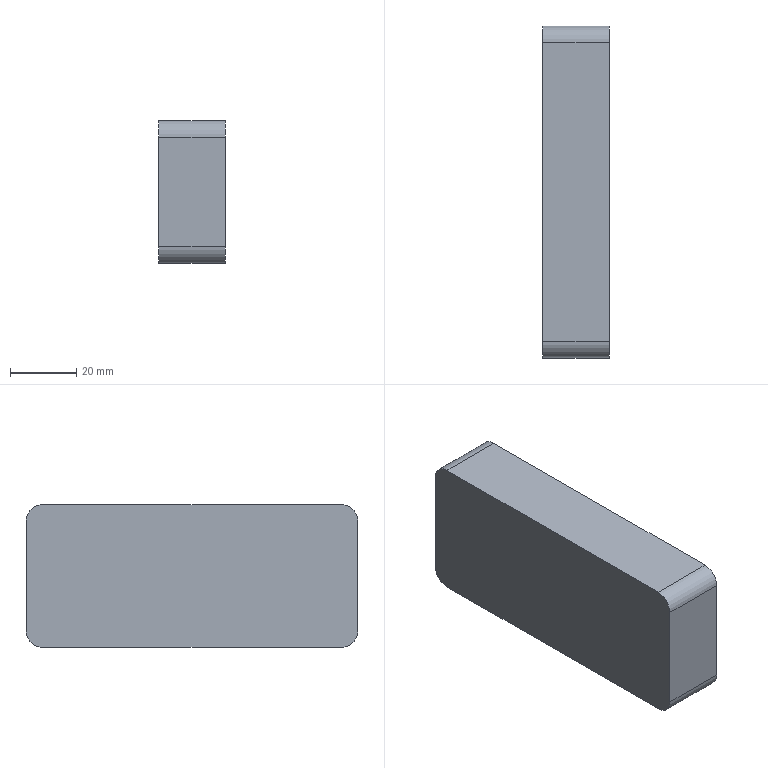Part | STEP file | 4-20.sldasm-Part-14 | 1 solid | 10 faces | box 20 x 100 x 43 mm | volume 85571 mm3 | plane 6 | cylinder 4 | commonest cylinder face diameters 10 x4
STEP:
#1=CARTESIAN_POINT('',(245.,464.25,-67.75));
#2=VERTEX_POINT('',#1);
#3=CARTESIAN_POINT('',(245.,374.25,-67.75));
#4=VERTEX_POINT('',#3);
#5=CARTESIAN_POINT('',(245.,464.25,-67.75));
#6=DIRECTION('',(0.,-1.,0.));
#7=VECTOR('',#6,1000.);
#8=LINE('',#5,#7);
#9=EDGE_CURVE('',#2,#4,#8,.T.);
#10=ORIENTED_EDGE('',*,*,#9,.T.);
#11=CARTESIAN_POINT('',(225.,374.25,-67.75));
#12=VERTEX_POINT('',#11);
#13=CARTESIAN_POINT('',(225.,374.25,-67.75));
#14=DIRECTION('',(1.,0.,0.));
#15=VECTOR('',#14,1000.);
#16=LINE('',#13,#15);
#17=EDGE_CURVE('',#12,#4,#16,.T.);
#18=ORIENTED_EDGE('',*,*,#17,.F.);
#19=CARTESIAN_POINT('',(225.,464.25,-67.75));
#20=VERTEX_POINT('',#19);
#21=CARTESIAN_POINT('',(225.,464.25,-67.75));
#22=DIRECTION('',(0.,-1.,0.));
#23=VECTOR('',#22,1000.);
#24=LINE('',#21,#23);
#25=EDGE_CURVE('',#20,#12,#24,.T.);
#26=ORIENTED_EDGE('',*,*,#25,.F.);
#27=CARTESIAN_POINT('',(225.,464.25,-67.75));
#28=DIRECTION('',(1.,0.,0.));
#29=VECTOR('',#28,1000.);
#30=LINE('',#27,#29);
#31=EDGE_CURVE('',#20,#2,#30,.T.);
#32=ORIENTED_EDGE('',*,*,#31,.T.);
#33=EDGE_LOOP('',(#10,#18,#26,#32));
#34=FACE_OUTER_BOUND('',#33,.T.);
#35=CARTESIAN_POINT('',(225.,464.25,-67.75));
#36=DIRECTION('',(0.,0.,1.));
#37=DIRECTION('',(0.,-1.,0.));
#38=AXIS2_PLACEMENT_3D('',#35,#36,#37);
#39=PLANE('',#38);
#40=ADVANCED_FACE('',(#34),#39,.F.);
#41=CARTESIAN_POINT('',(245.,369.25,-62.75));
#42=VERTEX_POINT('',#41);
#43=CARTESIAN_POINT('',(245.,374.25,-62.75));
#44=DIRECTION('',(-1.,0.,0.));
#45=DIRECTION('',(0.,0.,1.));
#46=AXIS2_PLACEMENT_3D('',#43,#44,#45);
#47=CIRCLE('',#46,5.);
#48=EDGE_CURVE('',#4,#42,#47,.T.);
#49=ORIENTED_EDGE('',*,*,#48,.T.);
#50=CARTESIAN_POINT('',(225.,369.25,-62.75));
#51=VERTEX_POINT('',#50);
#52=CARTESIAN_POINT('',(225.,369.25,-62.75));
#53=DIRECTION('',(1.,0.,0.));
#54=VECTOR('',#53,1000.);
#55=LINE('',#52,#54);
#56=EDGE_CURVE('',#51,#42,#55,.T.);
#57=ORIENTED_EDGE('',*,*,#56,.F.);
#58=CARTESIAN_POINT('',(225.,374.25,-62.75));
#59=DIRECTION('',(-1.,0.,0.));
#60=DIRECTION('',(0.,0.,1.));
#61=AXIS2_PLACEMENT_3D('',#58,#59,#60);
#62=CIRCLE('',#61,5.);
#63=EDGE_CURVE('',#12,#51,#62,.T.);
#64=ORIENTED_EDGE('',*,*,#63,.F.);
#65=ORIENTED_EDGE('',*,*,#17,.T.);
#66=EDGE_LOOP('',(#49,#57,#64,#65));
#67=FACE_OUTER_BOUND('',#66,.T.);
#68=CARTESIAN_POINT('',(225.,374.25,-62.75));
#69=DIRECTION('',(1.,0.,0.));
#70=DIRECTION('',(0.,1.,0.));
#71=AXIS2_PLACEMENT_3D('',#68,#69,#70);
#72=CYLINDRICAL_SURFACE('',#71,5.);
#73=ADVANCED_FACE('',(#67),#72,.T.);
#74=CARTESIAN_POINT('',(245.,369.25,-29.75));
#75=VERTEX_POINT('',#74);
#76=CARTESIAN_POINT('',(245.,369.25,-62.75));
#77=DIRECTION('',(0.,0.,1.));
#78=VECTOR('',#77,1000.);
#79=LINE('',#76,#78);
#80=EDGE_CURVE('',#42,#75,#79,.T.);
#81=ORIENTED_EDGE('',*,*,#80,.T.);
#82=CARTESIAN_POINT('',(225.,369.25,-29.75));
#83=VERTEX_POINT('',#82);
#84=CARTESIAN_POINT('',(225.,369.25,-29.75));
#85=DIRECTION('',(1.,0.,0.));
#86=VECTOR('',#85,1000.);
#87=LINE('',#84,#86);
#88=EDGE_CURVE('',#83,#75,#87,.T.);
#89=ORIENTED_EDGE('',*,*,#88,.F.);
#90=CARTESIAN_POINT('',(225.,369.25,-62.75));
#91=DIRECTION('',(0.,0.,1.));
#92=VECTOR('',#91,1000.);
#93=LINE('',#90,#92);
#94=EDGE_CURVE('',#51,#83,#93,.T.);
#95=ORIENTED_EDGE('',*,*,#94,.F.);
#96=ORIENTED_EDGE('',*,*,#56,.T.);
#97=EDGE_LOOP('',(#81,#89,#95,#96));
#98=FACE_OUTER_BOUND('',#97,.T.);
#99=CARTESIAN_POINT('',(225.,369.25,-62.75));
#100=DIRECTION('',(0.,1.,0.));
#101=DIRECTION('',(-1.,0.,0.));
#102=AXIS2_PLACEMENT_3D('',#99,#100,#101);
#103=PLANE('',#102);
#104=ADVANCED_FACE('',(#98),#103,.F.);
#105=CARTESIAN_POINT('',(245.,374.25,-24.75));
#106=VERTEX_POINT('',#105);
#107=CARTESIAN_POINT('',(245.,374.25,-29.75));
#108=DIRECTION('',(-1.,0.,0.));
#109=DIRECTION('',(0.,0.,1.));
#110=AXIS2_PLACEMENT_3D('',#107,#108,#109);
#111=CIRCLE('',#110,5.);
#112=EDGE_CURVE('',#75,#106,#111,.T.);
#113=ORIENTED_EDGE('',*,*,#112,.T.);
#114=CARTESIAN_POINT('',(225.,374.25,-24.75));
#115=VERTEX_POINT('',#114);
#116=CARTESIAN_POINT('',(225.,374.25,-24.75));
#117=DIRECTION('',(1.,0.,0.));
#118=VECTOR('',#117,1000.);
#119=LINE('',#116,#118);
#120=EDGE_CURVE('',#115,#106,#119,.T.);
#121=ORIENTED_EDGE('',*,*,#120,.F.);
#122=CARTESIAN_POINT('',(225.,374.25,-29.75));
#123=DIRECTION('',(-1.,0.,0.));
#124=DIRECTION('',(0.,0.,1.));
#125=AXIS2_PLACEMENT_3D('',#122,#123,#124);
#126=CIRCLE('',#125,5.);
#127=EDGE_CURVE('',#83,#115,#126,.T.);
#128=ORIENTED_EDGE('',*,*,#127,.F.);
#129=ORIENTED_EDGE('',*,*,#88,.T.);
#130=EDGE_LOOP('',(#113,#121,#128,#129));
#131=FACE_OUTER_BOUND('',#130,.T.);
#132=CARTESIAN_POINT('',(225.,374.25,-29.75));
#133=DIRECTION('',(1.,0.,0.));
#134=DIRECTION('',(0.,1.,0.));
#135=AXIS2_PLACEMENT_3D('',#132,#133,#134);
#136=CYLINDRICAL_SURFACE('',#135,5.);
#137=ADVANCED_FACE('',(#131),#136,.T.);
#138=CARTESIAN_POINT('',(245.,464.25,-24.75));
#139=VERTEX_POINT('',#138);
#140=CARTESIAN_POINT('',(245.,374.25,-24.75));
#141=DIRECTION('',(0.,1.,0.));
#142=VECTOR('',#141,1000.);
#143=LINE('',#140,#142);
#144=EDGE_CURVE('',#106,#139,#143,.T.);
#145=ORIENTED_EDGE('',*,*,#144,.T.);
#146=CARTESIAN_POINT('',(225.,464.25,-24.75));
#147=VERTEX_POINT('',#146);
#148=CARTESIAN_POINT('',(225.,464.25,-24.75));
#149=DIRECTION('',(1.,0.,0.));
#150=VECTOR('',#149,1000.);
#151=LINE('',#148,#150);
#152=EDGE_CURVE('',#147,#139,#151,.T.);
#153=ORIENTED_EDGE('',*,*,#152,.F.);
#154=CARTESIAN_POINT('',(225.,374.25,-24.75));
#155=DIRECTION('',(0.,1.,0.));
#156=VECTOR('',#155,1000.);
#157=LINE('',#154,#156);
#158=EDGE_CURVE('',#115,#147,#157,.T.);
#159=ORIENTED_EDGE('',*,*,#158,.F.);
#160=ORIENTED_EDGE('',*,*,#120,.T.);
#161=EDGE_LOOP('',(#145,#153,#159,#160));
#162=FACE_OUTER_BOUND('',#161,.T.);
#163=CARTESIAN_POINT('',(225.,374.25,-24.75));
#164=DIRECTION('',(0.,0.,-1.));
#165=DIRECTION('',(0.,1.,0.));
#166=AXIS2_PLACEMENT_3D('',#163,#164,#165);
#167=PLANE('',#166);
#168=ADVANCED_FACE('',(#162),#167,.F.);
#169=CARTESIAN_POINT('',(245.,469.25,-29.75));
#170=VERTEX_POINT('',#169);
#171=CARTESIAN_POINT('',(245.,464.25,-29.75));
#172=DIRECTION('',(-1.,0.,0.));
#173=DIRECTION('',(0.,0.,1.));
#174=AXIS2_PLACEMENT_3D('',#171,#172,#173);
#175=CIRCLE('',#174,5.);
#176=EDGE_CURVE('',#139,#170,#175,.T.);
#177=ORIENTED_EDGE('',*,*,#176,.T.);
#178=CARTESIAN_POINT('',(225.,469.25,-29.75));
#179=VERTEX_POINT('',#178);
#180=CARTESIAN_POINT('',(225.,469.25,-29.75));
#181=DIRECTION('',(1.,0.,0.));
#182=VECTOR('',#181,1000.);
#183=LINE('',#180,#182);
#184=EDGE_CURVE('',#179,#170,#183,.T.);
#185=ORIENTED_EDGE('',*,*,#184,.F.);
#186=CARTESIAN_POINT('',(225.,464.25,-29.75));
#187=DIRECTION('',(-1.,0.,0.));
#188=DIRECTION('',(0.,0.,1.));
#189=AXIS2_PLACEMENT_3D('',#186,#187,#188);
#190=CIRCLE('',#189,5.);
#191=EDGE_CURVE('',#147,#179,#190,.T.);
#192=ORIENTED_EDGE('',*,*,#191,.F.);
#193=ORIENTED_EDGE('',*,*,#152,.T.);
#194=EDGE_LOOP('',(#177,#185,#192,#193));
#195=FACE_OUTER_BOUND('',#194,.T.);
#196=CARTESIAN_POINT('',(225.,464.25,-29.75));
#197=DIRECTION('',(1.,0.,0.));
#198=DIRECTION('',(0.,1.,0.));
#199=AXIS2_PLACEMENT_3D('',#196,#197,#198);
#200=CYLINDRICAL_SURFACE('',#199,5.);
#201=ADVANCED_FACE('',(#195),#200,.T.);
#202=CARTESIAN_POINT('',(245.,469.25,-62.75));
#203=VERTEX_POINT('',#202);
#204=CARTESIAN_POINT('',(245.,469.25,-29.75));
#205=DIRECTION('',(0.,0.,-1.));
#206=VECTOR('',#205,1000.);
#207=LINE('',#204,#206);
#208=EDGE_CURVE('',#170,#203,#207,.T.);
#209=ORIENTED_EDGE('',*,*,#208,.T.);
#210=CARTESIAN_POINT('',(225.,469.25,-62.75));
#211=VERTEX_POINT('',#210);
#212=CARTESIAN_POINT('',(225.,469.25,-62.75));
#213=DIRECTION('',(1.,0.,0.));
#214=VECTOR('',#213,1000.);
#215=LINE('',#212,#214);
#216=EDGE_CURVE('',#211,#203,#215,.T.);
#217=ORIENTED_EDGE('',*,*,#216,.F.);
#218=CARTESIAN_POINT('',(225.,469.25,-29.75));
#219=DIRECTION('',(0.,0.,-1.));
#220=VECTOR('',#219,1000.);
#221=LINE('',#218,#220);
#222=EDGE_CURVE('',#179,#211,#221,.T.);
#223=ORIENTED_EDGE('',*,*,#222,.F.);
#224=ORIENTED_EDGE('',*,*,#184,.T.);
#225=EDGE_LOOP('',(#209,#217,#223,#224));
#226=FACE_OUTER_BOUND('',#225,.T.);
#227=CARTESIAN_POINT('',(225.,469.25,-29.75));
#228=DIRECTION('',(0.,-1.,0.));
#229=DIRECTION('',(0.,0.,-1.));
#230=AXIS2_PLACEMENT_3D('',#227,#228,#229);
#231=PLANE('',#230);
#232=ADVANCED_FACE('',(#226),#231,.F.);
#233=CARTESIAN_POINT('',(245.,464.25,-62.75));
#234=DIRECTION('',(-1.,0.,0.));
#235=DIRECTION('',(0.,0.,1.));
#236=AXIS2_PLACEMENT_3D('',#233,#234,#235);
#237=CIRCLE('',#236,5.);
#238=EDGE_CURVE('',#203,#2,#237,.T.);
#239=ORIENTED_EDGE('',*,*,#238,.T.);
#240=ORIENTED_EDGE('',*,*,#31,.F.);
#241=CARTESIAN_POINT('',(225.,464.25,-62.75));
#242=DIRECTION('',(-1.,0.,0.));
#243=DIRECTION('',(0.,0.,1.));
#244=AXIS2_PLACEMENT_3D('',#241,#242,#243);
#245=CIRCLE('',#244,5.);
#246=EDGE_CURVE('',#211,#20,#245,.T.);
#247=ORIENTED_EDGE('',*,*,#246,.F.);
#248=ORIENTED_EDGE('',*,*,#216,.T.);
#249=EDGE_LOOP('',(#239,#240,#247,#248));
#250=FACE_OUTER_BOUND('',#249,.T.);
#251=CARTESIAN_POINT('',(225.,464.25,-62.75));
#252=DIRECTION('',(1.,0.,0.));
#253=DIRECTION('',(0.,1.,0.));
#254=AXIS2_PLACEMENT_3D('',#251,#252,#253);
#255=CYLINDRICAL_SURFACE('',#254,5.);
#256=ADVANCED_FACE('',(#250),#255,.T.);
#257=ORIENTED_EDGE('',*,*,#25,.T.);
#258=ORIENTED_EDGE('',*,*,#63,.T.);
#259=ORIENTED_EDGE('',*,*,#94,.T.);
#260=ORIENTED_EDGE('',*,*,#127,.T.);
#261=ORIENTED_EDGE('',*,*,#158,.T.);
#262=ORIENTED_EDGE('',*,*,#191,.T.);
#263=ORIENTED_EDGE('',*,*,#222,.T.);
#264=ORIENTED_EDGE('',*,*,#246,.T.);
#265=EDGE_LOOP('',(#257,#258,#259,#260,#261,#262,#263,#264));
#266=FACE_OUTER_BOUND('',#265,.T.);
#267=CARTESIAN_POINT('',(225.,374.25,-62.75));
#268=DIRECTION('',(-1.,0.,0.));
#269=DIRECTION('',(0.,-1.,0.));
#270=AXIS2_PLACEMENT_3D('',#267,#268,#269);
#271=PLANE('',#270);
#272=ADVANCED_FACE('',(#266),#271,.T.);
#273=ORIENTED_EDGE('',*,*,#9,.F.);
#274=ORIENTED_EDGE('',*,*,#238,.F.);
#275=ORIENTED_EDGE('',*,*,#208,.F.);
#276=ORIENTED_EDGE('',*,*,#176,.F.);
#277=ORIENTED_EDGE('',*,*,#144,.F.);
#278=ORIENTED_EDGE('',*,*,#112,.F.);
#279=ORIENTED_EDGE('',*,*,#80,.F.);
#280=ORIENTED_EDGE('',*,*,#48,.F.);
#281=EDGE_LOOP('',(#273,#274,#275,#276,#277,#278,#279,#280));
#282=FACE_OUTER_BOUND('',#281,.T.);
#283=CARTESIAN_POINT('',(245.,374.25,-62.75));
#284=DIRECTION('',(-1.,0.,0.));
#285=DIRECTION('',(0.,-1.,0.));
#286=AXIS2_PLACEMENT_3D('',#283,#284,#285);
#287=PLANE('',#286);
#288=ADVANCED_FACE('',(#282),#287,.F.);
#289=CLOSED_SHELL('',(#40,#73,#104,#137,#168,#201,#232,#256,#272,#288));
#290=MANIFOLD_SOLID_BREP('',#289);
#291=CARTESIAN_POINT('',(0.,0.,0.));
#292=DIRECTION('',(0.,0.,1.));
#293=DIRECTION('',(1.,0.,0.));
#294=AXIS2_PLACEMENT_3D('',#291,#292,#293);
#295=(LENGTH_UNIT()NAMED_UNIT(*)SI_UNIT(.MILLI.,.METRE.));
#296=UNCERTAINTY_MEASURE_WITH_UNIT(LENGTH_MEASURE(0.00001),#295,'','');
#297=(NAMED_UNIT(*)PLANE_ANGLE_UNIT()SI_UNIT($,.RADIAN.));
#298=(NAMED_UNIT(*)SI_UNIT($,.STERADIAN.)SOLID_ANGLE_UNIT());
#299=(GEOMETRIC_REPRESENTATION_CONTEXT(3)GLOBAL_UNCERTAINTY_ASSIGNED_CONTEXT((#296))GLOBAL_UNIT_ASSIGNED_CONTEXT((#295,#297,#298))REPRESENTATION_CONTEXT('',''));
#300=ADVANCED_BREP_SHAPE_REPRESENTATION('',(#290,#294),#299);